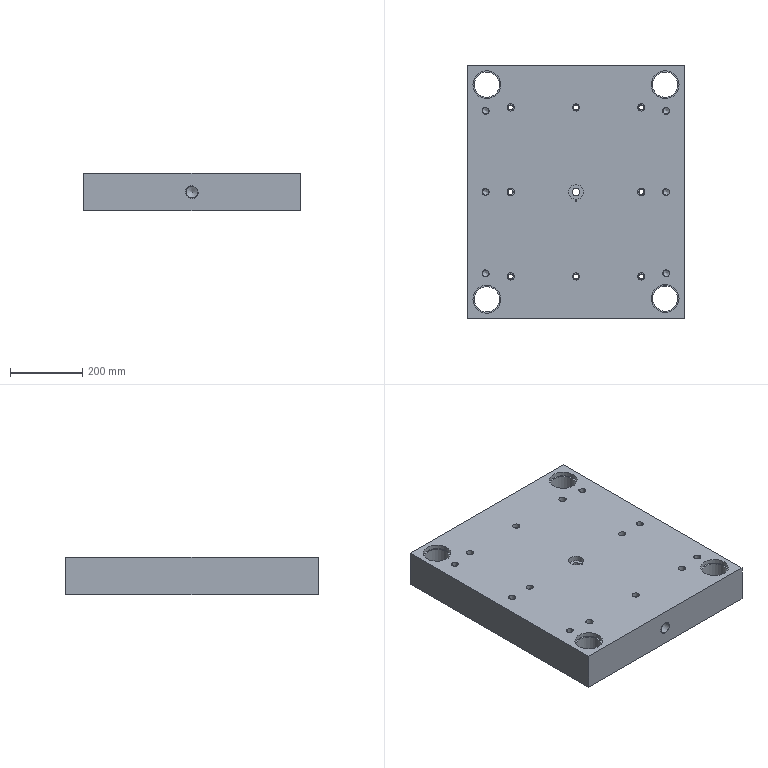Part | NX | features 模具.stp<1>[5] 2 | 1 solid | 154 faces | box 600 x 700 x 105 mm | volume 28538316 mm3 | plane 76 | cylinder 70 | cone 8 | commonest cylinder face diameters 20 x14 12 x8 14 x8 17.5 x6 19.7 x6 24 x6